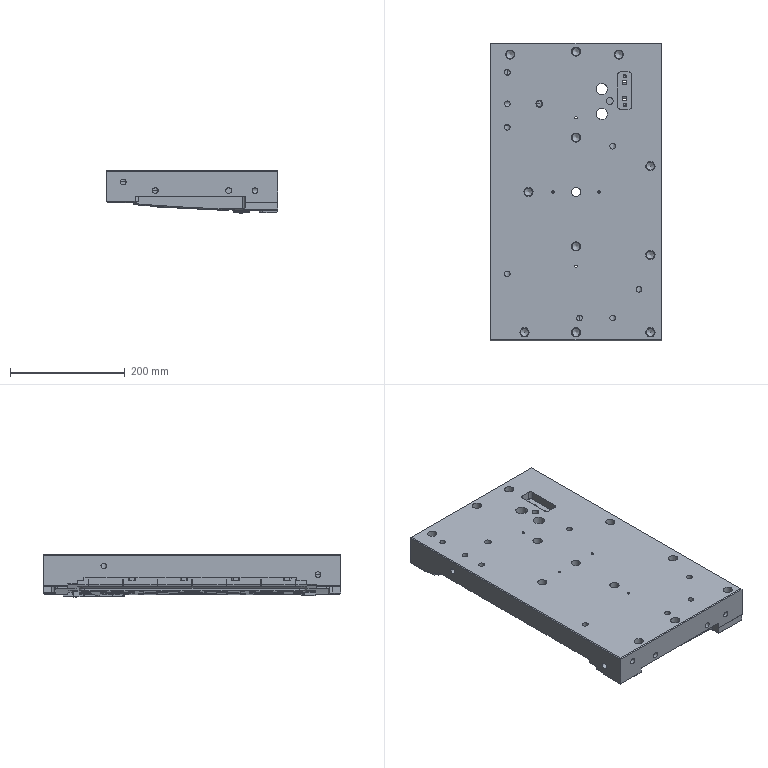Part | STEP file | solid 207 | 1 solid | 1132 faces | box 300 x 520 x 75.001 mm | volume 8769898 mm3 | plane 600 | cylinder 348 | spline 105 | torus 37 | cone 24 | sphere 12 | other 6 | commonest cylinder face diameters 0.603 x51 10 x40 7.8 x36 8 x29 1.004 x26 4.02 x22